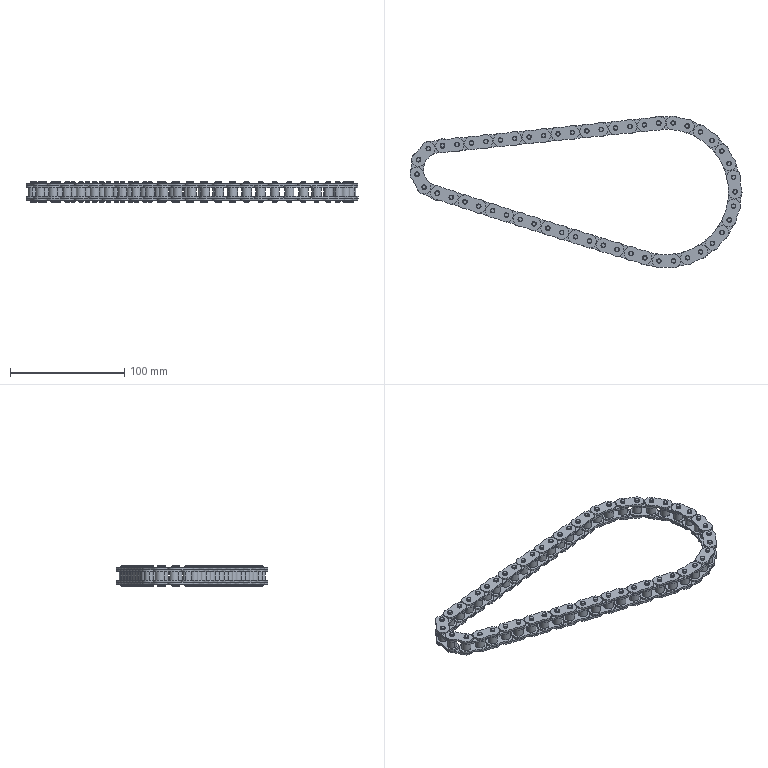Part | SolidWorks | features BaseBody 78 | 78 solids | 1560 faces | box 290.935 x 132.94 x 17.8 mm | volume 66914 mm3 | cylinder 1040 | plane 312 | cone 208 | commonest cylinder face diameters 3.98 x416 12.07 x312 55.348 x208 7.92 x104